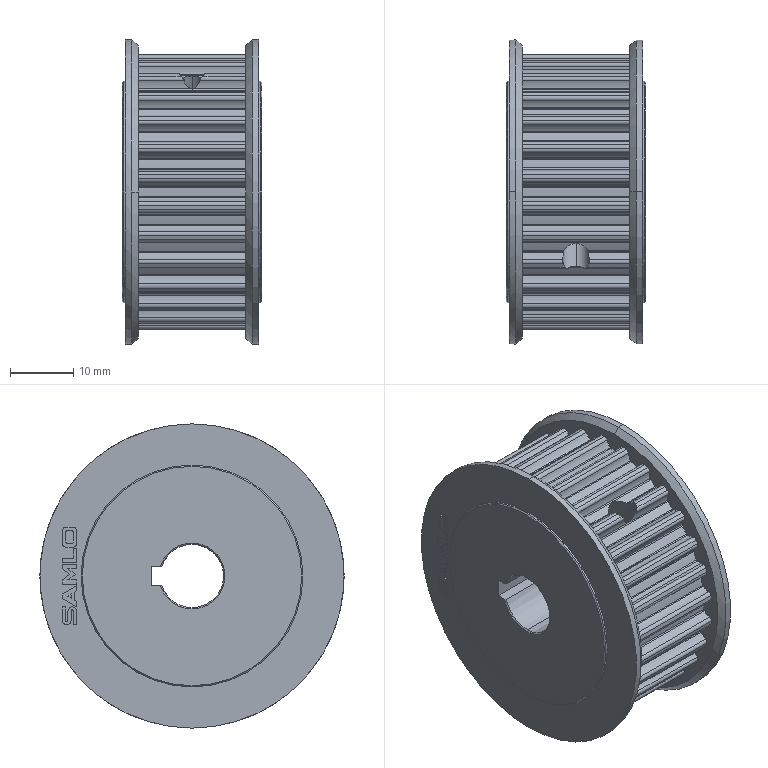Part | SolidWorks | features BaseBody 1 | 1 solid | 367 faces | box 22 x 48 x 48 mm | volume 28934 mm3 | cylinder 289 | plane 64 | cone 14 | commonest cylinder face diameters 1.1 x70 0.5 x68 6.55 x63 40.06 x30 43.6 x29 0.523 x4